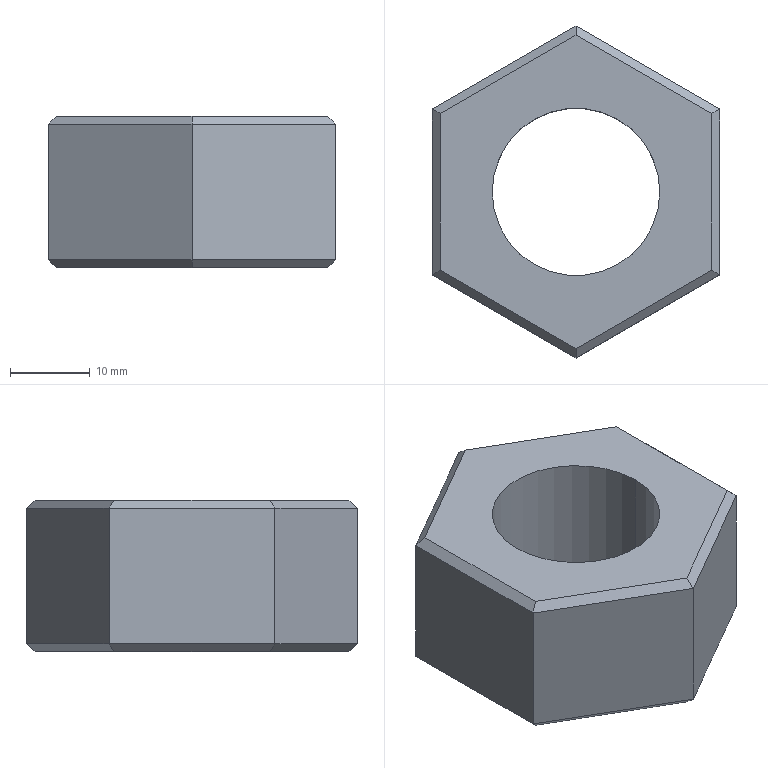Part | STEP file | GLSJ-10-36 | 1 solid | 22 faces | box 36 x 41.569 x 19 mm | volume 14622 mm3 | plane 20 | cylinder 2 | commonest cylinder face diameters 21 x2
STEP:
#1=CARTESIAN_POINT('',(0.,0.,0.));
#2=DIRECTION('',(0.,0.,1.));
#3=DIRECTION('',(1.,0.,0.));
#4=AXIS2_PLACEMENT_3D('',#1,#2,#3);
#5=CARTESIAN_POINT('',(10.5,0.,0.));
#6=VERTEX_POINT('',#5);
#7=CARTESIAN_POINT('',(10.5,0.,19.));
#8=VERTEX_POINT('',#7);
#9=CARTESIAN_POINT('',(10.5,0.,19.));
#10=DIRECTION('',(0.,0.,1.));
#11=VECTOR('',#10,1.);
#12=LINE('',#9,#11);
#13=CARTESIAN_POINT('',(0.,0.,19.));
#14=DIRECTION('',(0.,0.,1.));
#15=DIRECTION('',(1.,0.,0.));
#16=AXIS2_PLACEMENT_3D('',#13,#14,#15);
#17=CYLINDRICAL_SURFACE('',#16,10.5);
#18=CARTESIAN_POINT('',(6.283,0.));
#19=DIRECTION('',(0.,1.));
#20=VECTOR('',#19,1.);
#21=LINE('',#18,#20);
#22=(GEOMETRIC_REPRESENTATION_CONTEXT(2)PARAMETRIC_REPRESENTATION_CONTEXT()REPRESENTATION_CONTEXT('',''));
#23=DEFINITIONAL_REPRESENTATION('',(#21),#22);
#24=PCURVE('',#17,#23);
#25=CARTESIAN_POINT('',(0.,0.,19.));
#26=DIRECTION('',(0.,0.,1.));
#27=DIRECTION('',(1.,0.,0.));
#28=AXIS2_PLACEMENT_3D('',#25,#26,#27);
#29=CYLINDRICAL_SURFACE('',#28,10.5);
#30=CARTESIAN_POINT('',(0.,0.));
#31=DIRECTION('',(0.,1.));
#32=VECTOR('',#31,1.);
#33=LINE('',#30,#32);
#34=(GEOMETRIC_REPRESENTATION_CONTEXT(2)PARAMETRIC_REPRESENTATION_CONTEXT()REPRESENTATION_CONTEXT('',''));
#35=DEFINITIONAL_REPRESENTATION('',(#33),#34);
#36=PCURVE('',#29,#35);
#37=SURFACE_CURVE('',#12,(#24,#36),.PCURVE_S1.);
#38=EDGE_CURVE('',#6,#8,#37,.T.);
#39=ORIENTED_EDGE('',*,*,#38,.T.);
#40=CARTESIAN_POINT('',(-10.5,0.,19.));
#41=VERTEX_POINT('',#40);
#42=CARTESIAN_POINT('',(0.,0.,19.));
#43=DIRECTION('',(0.,0.,1.));
#44=DIRECTION('',(1.,0.,0.));
#45=AXIS2_PLACEMENT_3D('',#42,#43,#44);
#46=CIRCLE('',#45,10.5);
#47=CARTESIAN_POINT('',(0.,0.));
#48=DIRECTION('',(1.,0.));
#49=VECTOR('',#48,1.);
#50=LINE('',#47,#49);
#51=(GEOMETRIC_REPRESENTATION_CONTEXT(2)PARAMETRIC_REPRESENTATION_CONTEXT()REPRESENTATION_CONTEXT('',''));
#52=DEFINITIONAL_REPRESENTATION('',(#50),#51);
#53=PCURVE('',#17,#52);
#54=CARTESIAN_POINT('',(0.,0.,19.));
#55=DIRECTION('',(0.,0.,1.));
#56=DIRECTION('',(1.,0.,0.));
#57=AXIS2_PLACEMENT_3D('',#54,#55,#56);
#58=PLANE('',#57);
#59=CARTESIAN_POINT('',(0.,0.));
#60=DIRECTION('',(1.,0.));
#61=AXIS2_PLACEMENT_2D('',#59,#60);
#62=CIRCLE('',#61,10.5);
#63=(GEOMETRIC_REPRESENTATION_CONTEXT(2)PARAMETRIC_REPRESENTATION_CONTEXT()REPRESENTATION_CONTEXT('',''));
#64=DEFINITIONAL_REPRESENTATION('',(#62),#63);
#65=PCURVE('',#58,#64);
#66=SURFACE_CURVE('',#46,(#53,#65),.PCURVE_S1.);
#67=EDGE_CURVE('',#41,#8,#66,.T.);
#68=ORIENTED_EDGE('',*,*,#67,.F.);
#69=CARTESIAN_POINT('',(-10.5,0.,0.));
#70=VERTEX_POINT('',#69);
#71=CARTESIAN_POINT('',(-10.5,0.,19.));
#72=DIRECTION('',(0.,0.,1.));
#73=VECTOR('',#72,1.);
#74=LINE('',#71,#73);
#75=CARTESIAN_POINT('',(3.142,0.));
#76=DIRECTION('',(0.,1.));
#77=VECTOR('',#76,1.);
#78=LINE('',#75,#77);
#79=(GEOMETRIC_REPRESENTATION_CONTEXT(2)PARAMETRIC_REPRESENTATION_CONTEXT()REPRESENTATION_CONTEXT('',''));
#80=DEFINITIONAL_REPRESENTATION('',(#78),#79);
#81=PCURVE('',#17,#80);
#82=CARTESIAN_POINT('',(3.142,0.));
#83=DIRECTION('',(0.,1.));
#84=VECTOR('',#83,1.);
#85=LINE('',#82,#84);
#86=(GEOMETRIC_REPRESENTATION_CONTEXT(2)PARAMETRIC_REPRESENTATION_CONTEXT()REPRESENTATION_CONTEXT('',''));
#87=DEFINITIONAL_REPRESENTATION('',(#85),#86);
#88=PCURVE('',#29,#87);
#89=SURFACE_CURVE('',#74,(#81,#88),.PCURVE_S1.);
#90=EDGE_CURVE('',#70,#41,#89,.T.);
#91=ORIENTED_EDGE('',*,*,#90,.F.);
#92=CARTESIAN_POINT('',(0.,0.,0.));
#93=DIRECTION('',(0.,0.,1.));
#94=DIRECTION('',(1.,0.,0.));
#95=AXIS2_PLACEMENT_3D('',#92,#93,#94);
#96=CIRCLE('',#95,10.5);
#97=CARTESIAN_POINT('',(0.,-19.));
#98=DIRECTION('',(1.,0.));
#99=VECTOR('',#98,1.);
#100=LINE('',#97,#99);
#101=(GEOMETRIC_REPRESENTATION_CONTEXT(2)PARAMETRIC_REPRESENTATION_CONTEXT()REPRESENTATION_CONTEXT('',''));
#102=DEFINITIONAL_REPRESENTATION('',(#100),#101);
#103=PCURVE('',#17,#102);
#104=CARTESIAN_POINT('',(0.,0.,0.));
#105=DIRECTION('',(0.,0.,1.));
#106=DIRECTION('',(1.,0.,0.));
#107=AXIS2_PLACEMENT_3D('',#104,#105,#106);
#108=PLANE('',#107);
#109=CARTESIAN_POINT('',(0.,0.));
#110=DIRECTION('',(1.,0.));
#111=AXIS2_PLACEMENT_2D('',#109,#110);
#112=CIRCLE('',#111,10.5);
#113=(GEOMETRIC_REPRESENTATION_CONTEXT(2)PARAMETRIC_REPRESENTATION_CONTEXT()REPRESENTATION_CONTEXT('',''));
#114=DEFINITIONAL_REPRESENTATION('',(#112),#113);
#115=PCURVE('',#108,#114);
#116=SURFACE_CURVE('',#96,(#103,#115),.PCURVE_S1.);
#117=EDGE_CURVE('',#70,#6,#116,.T.);
#118=ORIENTED_EDGE('',*,*,#117,.T.);
#119=EDGE_LOOP('',(#39,#68,#91,#118));
#120=FACE_BOUND('',#119,.F.);
#121=ADVANCED_FACE('',(#120),#17,.F.);
#122=CARTESIAN_POINT('',(-18.,10.392,18.));
#123=VERTEX_POINT('',#122);
#124=CARTESIAN_POINT('',(-18.,10.392,1.));
#125=VERTEX_POINT('',#124);
#126=CARTESIAN_POINT('',(-18.,10.392,19.));
#127=DIRECTION('',(0.,0.,-1.));
#128=VECTOR('',#127,1.);
#129=LINE('',#126,#128);
#130=CARTESIAN_POINT('',(-18.,10.392,19.));
#131=DIRECTION('',(1.,0.,0.));
#132=DIRECTION('',(0.,0.,-1.));
#133=AXIS2_PLACEMENT_3D('',#130,#131,#132);
#134=PLANE('',#133);
#135=CARTESIAN_POINT('',(0.,0.));
#136=DIRECTION('',(1.,0.));
#137=VECTOR('',#136,1.);
#138=LINE('',#135,#137);
#139=(GEOMETRIC_REPRESENTATION_CONTEXT(2)PARAMETRIC_REPRESENTATION_CONTEXT()REPRESENTATION_CONTEXT('',''));
#140=DEFINITIONAL_REPRESENTATION('',(#138),#139);
#141=PCURVE('',#134,#140);
#142=CARTESIAN_POINT('',(0.,20.785,19.));
#143=DIRECTION('',(0.5,-0.866,0.));
#144=DIRECTION('',(0.866,0.5,0.));
#145=AXIS2_PLACEMENT_3D('',#142,#143,#144);
#146=PLANE('',#145);
#147=CARTESIAN_POINT('',(-20.785,0.));
#148=DIRECTION('',(0.,-1.));
#149=VECTOR('',#148,1.);
#150=LINE('',#147,#149);
#151=(GEOMETRIC_REPRESENTATION_CONTEXT(2)PARAMETRIC_REPRESENTATION_CONTEXT()REPRESENTATION_CONTEXT('',''));
#152=DEFINITIONAL_REPRESENTATION('',(#150),#151);
#153=PCURVE('',#146,#152);
#154=SURFACE_CURVE('',#129,(#141,#153),.PCURVE_S1.);
#155=EDGE_CURVE('',#123,#125,#154,.T.);
#156=ORIENTED_EDGE('',*,*,#155,.T.);
#157=CARTESIAN_POINT('',(-18.,-10.392,1.));
#158=VERTEX_POINT('',#157);
#159=CARTESIAN_POINT('',(-18.,10.392,1.));
#160=DIRECTION('',(0.,-1.,0.));
#161=VECTOR('',#160,1.);
#162=LINE('',#159,#161);
#163=CARTESIAN_POINT('',(18.,0.));
#164=DIRECTION('',(0.,-1.));
#165=VECTOR('',#164,1.);
#166=LINE('',#163,#165);
#167=(GEOMETRIC_REPRESENTATION_CONTEXT(2)PARAMETRIC_REPRESENTATION_CONTEXT()REPRESENTATION_CONTEXT('',''));
#168=DEFINITIONAL_REPRESENTATION('',(#166),#167);
#169=PCURVE('',#134,#168);
#170=CARTESIAN_POINT('',(-18.,10.392,1.));
#171=DIRECTION('',(0.7071,0.,0.7071));
#172=DIRECTION('',(0.,-1.,0.));
#173=AXIS2_PLACEMENT_3D('',#170,#171,#172);
#174=PLANE('',#173);
#175=CARTESIAN_POINT('',(0.,0.));
#176=DIRECTION('',(1.,0.));
#177=VECTOR('',#176,1.);
#178=LINE('',#175,#177);
#179=(GEOMETRIC_REPRESENTATION_CONTEXT(2)PARAMETRIC_REPRESENTATION_CONTEXT()REPRESENTATION_CONTEXT('',''));
#180=DEFINITIONAL_REPRESENTATION('',(#178),#179);
#181=PCURVE('',#174,#180);
#182=SURFACE_CURVE('',#162,(#169,#181),.PCURVE_S1.);
#183=EDGE_CURVE('',#125,#158,#182,.T.);
#184=ORIENTED_EDGE('',*,*,#183,.T.);
#185=CARTESIAN_POINT('',(-18.,-10.392,18.));
#186=VERTEX_POINT('',#185);
#187=CARTESIAN_POINT('',(-18.,-10.392,19.));
#188=DIRECTION('',(0.,0.,-1.));
#189=VECTOR('',#188,1.);
#190=LINE('',#187,#189);
#191=CARTESIAN_POINT('',(0.,-20.785));
#192=DIRECTION('',(1.,0.));
#193=VECTOR('',#192,1.);
#194=LINE('',#191,#193);
#195=(GEOMETRIC_REPRESENTATION_CONTEXT(2)PARAMETRIC_REPRESENTATION_CONTEXT()REPRESENTATION_CONTEXT('',''));
#196=DEFINITIONAL_REPRESENTATION('',(#194),#195);
#197=PCURVE('',#134,#196);
#198=CARTESIAN_POINT('',(-18.,-10.392,19.));
#199=DIRECTION('',(0.5,0.866,0.));
#200=DIRECTION('',(-0.866,0.5,0.));
#201=AXIS2_PLACEMENT_3D('',#198,#199,#200);
#202=PLANE('',#201);
#203=CARTESIAN_POINT('',(0.,0.));
#204=DIRECTION('',(0.,-1.));
#205=VECTOR('',#204,1.);
#206=LINE('',#203,#205);
#207=(GEOMETRIC_REPRESENTATION_CONTEXT(2)PARAMETRIC_REPRESENTATION_CONTEXT()REPRESENTATION_CONTEXT('',''));
#208=DEFINITIONAL_REPRESENTATION('',(#206),#207);
#209=PCURVE('',#202,#208);
#210=SURFACE_CURVE('',#190,(#197,#209),.PCURVE_S1.);
#211=EDGE_CURVE('',#186,#158,#210,.T.);
#212=ORIENTED_EDGE('',*,*,#211,.F.);
#213=CARTESIAN_POINT('',(-18.,10.392,18.));
#214=DIRECTION('',(0.,1.,0.));
#215=VECTOR('',#214,1.);
#216=LINE('',#213,#215);
#217=CARTESIAN_POINT('',(1.,0.));
#218=DIRECTION('',(0.,1.));
#219=VECTOR('',#218,1.);
#220=LINE('',#217,#219);
#221=(GEOMETRIC_REPRESENTATION_CONTEXT(2)PARAMETRIC_REPRESENTATION_CONTEXT()REPRESENTATION_CONTEXT('',''));
#222=DEFINITIONAL_REPRESENTATION('',(#220),#221);
#223=PCURVE('',#134,#222);
#224=CARTESIAN_POINT('',(-17.,0.,19.));
#225=DIRECTION('',(-0.7071,0.,0.7071));
#226=DIRECTION('',(0.,1.,0.));
#227=AXIS2_PLACEMENT_3D('',#224,#225,#226);
#228=PLANE('',#227);
#229=CARTESIAN_POINT('',(10.392,1.414));
#230=DIRECTION('',(1.,0.));
#231=VECTOR('',#230,1.);
#232=LINE('',#229,#231);
#233=(GEOMETRIC_REPRESENTATION_CONTEXT(2)PARAMETRIC_REPRESENTATION_CONTEXT()REPRESENTATION_CONTEXT('',''));
#234=DEFINITIONAL_REPRESENTATION('',(#232),#233);
#235=PCURVE('',#228,#234);
#236=SURFACE_CURVE('',#216,(#223,#235),.PCURVE_S1.);
#237=EDGE_CURVE('',#186,#123,#236,.T.);
#238=ORIENTED_EDGE('',*,*,#237,.T.);
#239=EDGE_LOOP('',(#156,#184,#212,#238));
#240=FACE_BOUND('',#239,.T.);
#241=ADVANCED_FACE('',(#240),#134,.F.);
#242=ORIENTED_EDGE('',*,*,#211,.T.);
#243=CARTESIAN_POINT('',(0.,-20.785,1.));
#244=VERTEX_POINT('',#243);
#245=CARTESIAN_POINT('',(-18.,-10.392,1.));
#246=DIRECTION('',(0.866,-0.5,0.));
#247=VECTOR('',#246,1.);
#248=LINE('',#245,#247);
#249=CARTESIAN_POINT('',(0.,-18.));
#250=DIRECTION('',(-1.,0.));
#251=VECTOR('',#250,1.);
#252=LINE('',#249,#251);
#253=(GEOMETRIC_REPRESENTATION_CONTEXT(2)PARAMETRIC_REPRESENTATION_CONTEXT()REPRESENTATION_CONTEXT('',''));
#254=DEFINITIONAL_REPRESENTATION('',(#252),#253);
#255=PCURVE('',#202,#254);
#256=CARTESIAN_POINT('',(-18.,-10.392,1.));
#257=DIRECTION('',(0.3536,0.6124,0.7071));
#258=DIRECTION('',(0.866,-0.5,0.));
#259=AXIS2_PLACEMENT_3D('',#256,#257,#258);
#260=PLANE('',#259);
#261=CARTESIAN_POINT('',(0.,0.));
#262=DIRECTION('',(1.,0.));
#263=VECTOR('',#262,1.);
#264=LINE('',#261,#263);
#265=(GEOMETRIC_REPRESENTATION_CONTEXT(2)PARAMETRIC_REPRESENTATION_CONTEXT()REPRESENTATION_CONTEXT('',''));
#266=DEFINITIONAL_REPRESENTATION('',(#264),#265);
#267=PCURVE('',#260,#266);
#268=SURFACE_CURVE('',#248,(#255,#267),.PCURVE_S1.);
#269=EDGE_CURVE('',#158,#244,#268,.T.);
#270=ORIENTED_EDGE('',*,*,#269,.T.);
#271=CARTESIAN_POINT('',(0.,-20.785,18.));
#272=VERTEX_POINT('',#271);
#273=CARTESIAN_POINT('',(0.,-20.785,19.));
#274=DIRECTION('',(0.,0.,-1.));
#275=VECTOR('',#274,1.);
#276=LINE('',#273,#275);
#277=CARTESIAN_POINT('',(-20.785,0.));
#278=DIRECTION('',(0.,-1.));
#279=VECTOR('',#278,1.);
#280=LINE('',#277,#279);
#281=(GEOMETRIC_REPRESENTATION_CONTEXT(2)PARAMETRIC_REPRESENTATION_CONTEXT()REPRESENTATION_CONTEXT('',''));
#282=DEFINITIONAL_REPRESENTATION('',(#280),#281);
#283=PCURVE('',#202,#282);
#284=CARTESIAN_POINT('',(0.,-20.785,19.));
#285=DIRECTION('',(-0.5,0.866,0.));
#286=DIRECTION('',(-0.866,-0.5,0.));
#287=AXIS2_PLACEMENT_3D('',#284,#285,#286);
#288=PLANE('',#287);
#289=CARTESIAN_POINT('',(0.,0.));
#290=DIRECTION('',(0.,-1.));
#291=VECTOR('',#290,1.);
#292=LINE('',#289,#291);
#293=(GEOMETRIC_REPRESENTATION_CONTEXT(2)PARAMETRIC_REPRESENTATION_CONTEXT()REPRESENTATION_CONTEXT('',''));
#294=DEFINITIONAL_REPRESENTATION('',(#292),#293);
#295=PCURVE('',#288,#294);
#296=SURFACE_CURVE('',#276,(#283,#295),.PCURVE_S1.);
#297=EDGE_CURVE('',#272,#244,#296,.T.);
#298=ORIENTED_EDGE('',*,*,#297,.F.);
#299=CARTESIAN_POINT('',(-18.,-10.392,18.));
#300=DIRECTION('',(-0.866,0.5,0.));
#301=VECTOR('',#300,1.);
#302=LINE('',#299,#301);
#303=CARTESIAN_POINT('',(0.,-1.));
#304=DIRECTION('',(1.,0.));
#305=VECTOR('',#304,1.);
#306=LINE('',#303,#305);
#307=(GEOMETRIC_REPRESENTATION_CONTEXT(2)PARAMETRIC_REPRESENTATION_CONTEXT()REPRESENTATION_CONTEXT('',''));
#308=DEFINITIONAL_REPRESENTATION('',(#306),#307);
#309=PCURVE('',#202,#308);
#310=CARTESIAN_POINT('',(-8.5,-14.722,19.));
#311=DIRECTION('',(-0.3536,-0.6124,0.7071));
#312=DIRECTION('',(-0.866,0.5,0.));
#313=AXIS2_PLACEMENT_3D('',#310,#311,#312);
#314=PLANE('',#313);
#315=CARTESIAN_POINT('',(10.392,1.414));
#316=DIRECTION('',(1.,0.));
#317=VECTOR('',#316,1.);
#318=LINE('',#315,#317);
#319=(GEOMETRIC_REPRESENTATION_CONTEXT(2)PARAMETRIC_REPRESENTATION_CONTEXT()REPRESENTATION_CONTEXT('',''));
#320=DEFINITIONAL_REPRESENTATION('',(#318),#319);
#321=PCURVE('',#314,#320);
#322=SURFACE_CURVE('',#302,(#309,#321),.PCURVE_S1.);
#323=EDGE_CURVE('',#272,#186,#322,.T.);
#324=ORIENTED_EDGE('',*,*,#323,.T.);
#325=EDGE_LOOP('',(#242,#270,#298,#324));
#326=FACE_BOUND('',#325,.T.);
#327=ADVANCED_FACE('',(#326),#202,.F.);
#328=ORIENTED_EDGE('',*,*,#297,.T.);
#329=CARTESIAN_POINT('',(18.,-10.392,1.));
#330=VERTEX_POINT('',#329);
#331=CARTESIAN_POINT('',(0.,-20.785,1.));
#332=DIRECTION('',(0.866,0.5,0.));
#333=VECTOR('',#332,1.);
#334=LINE('',#331,#333);
#335=CARTESIAN_POINT('',(0.,-18.));
#336=DIRECTION('',(-1.,0.));
#337=VECTOR('',#336,1.);
#338=LINE('',#335,#337);
#339=(GEOMETRIC_REPRESENTATION_CONTEXT(2)PARAMETRIC_REPRESENTATION_CONTEXT()REPRESENTATION_CONTEXT('',''));
#340=DEFINITIONAL_REPRESENTATION('',(#338),#339);
#341=PCURVE('',#288,#340);
#342=CARTESIAN_POINT('',(0.,-20.785,1.));
#343=DIRECTION('',(-0.3536,0.6124,0.7071));
#344=DIRECTION('',(0.866,0.5,0.));
#345=AXIS2_PLACEMENT_3D('',#342,#343,#344);
#346=PLANE('',#345);
#347=CARTESIAN_POINT('',(0.,0.));
#348=DIRECTION('',(1.,0.));
#349=VECTOR('',#348,1.);
#350=LINE('',#347,#349);
#351=(GEOMETRIC_REPRESENTATION_CONTEXT(2)PARAMETRIC_REPRESENTATION_CONTEXT()REPRESENTATION_CONTEXT('',''));
#352=DEFINITIONAL_REPRESENTATION('',(#350),#351);
#353=PCURVE('',#346,#352);
#354=SURFACE_CURVE('',#334,(#341,#353),.PCURVE_S1.);
#355=EDGE_CURVE('',#244,#330,#354,.T.);
#356=ORIENTED_EDGE('',*,*,#355,.T.);
#357=CARTESIAN_POINT('',(18.,-10.392,18.));
#358=VERTEX_POINT('',#357);
#359=CARTESIAN_POINT('',(18.,-10.392,19.));
#360=DIRECTION('',(0.,0.,-1.));
#361=VECTOR('',#360,1.);
#362=LINE('',#359,#361);
#363=CARTESIAN_POINT('',(-20.785,0.));
#364=DIRECTION('',(0.,-1.));
#365=VECTOR('',#364,1.);
#366=LINE('',#363,#365);
#367=(GEOMETRIC_REPRESENTATION_CONTEXT(2)PARAMETRIC_REPRESENTATION_CONTEXT()REPRESENTATION_CONTEXT('',''));
#368=DEFINITIONAL_REPRESENTATION('',(#366),#367);
#369=PCURVE('',#288,#368);
#370=CARTESIAN_POINT('',(18.,-10.392,19.));
#371=DIRECTION('',(-1.,0.,0.));
#372=DIRECTION('',(0.,-1.,0.));
#373=AXIS2_PLACEMENT_3D('',#370,#371,#372);
#374=PLANE('',#373);
#375=CARTESIAN_POINT('',(0.,0.));
#376=DIRECTION('',(0.,-1.));
#377=VECTOR('',#376,1.);
#378=LINE('',#375,#377);
#379=(GEOMETRIC_REPRESENTATION_CONTEXT(2)PARAMETRIC_REPRESENTATION_CONTEXT()REPRESENTATION_CONTEXT('',''));
#380=DEFINITIONAL_REPRESENTATION('',(#378),#379);
#381=PCURVE('',#374,#380);
#382=SURFACE_CURVE('',#362,(#369,#381),.PCURVE_S1.);
#383=EDGE_CURVE('',#358,#330,#382,.T.);
#384=ORIENTED_EDGE('',*,*,#383,.F.);
#385=CARTESIAN_POINT('',(0.,-20.785,18.));
#386=DIRECTION('',(-0.866,-0.5,0.));
#387=VECTOR('',#386,1.);
#388=LINE('',#385,#387);
#389=CARTESIAN_POINT('',(0.,-1.));
#390=DIRECTION('',(1.,0.));
#391=VECTOR('',#390,1.);
#392=LINE('',#389,#391);
#393=(GEOMETRIC_REPRESENTATION_CONTEXT(2)PARAMETRIC_REPRESENTATION_CONTEXT()REPRESENTATION_CONTEXT('',''));
#394=DEFINITIONAL_REPRESENTATION('',(#392),#393);
#395=PCURVE('',#288,#394);
#396=CARTESIAN_POINT('',(8.5,-14.722,19.));
#397=DIRECTION('',(0.3536,-0.6124,0.7071));
#398=DIRECTION('',(-0.866,-0.5,0.));
#399=AXIS2_PLACEMENT_3D('',#396,#397,#398);
#400=PLANE('',#399);
#401=CARTESIAN_POINT('',(10.392,1.414));
#402=DIRECTION('',(1.,0.));
#403=VECTOR('',#402,1.);
#404=LINE('',#401,#403);
#405=(GEOMETRIC_REPRESENTATION_CONTEXT(2)PARAMETRIC_REPRESENTATION_CONTEXT()REPRESENTATION_CONTEXT('',''));
#406=DEFINITIONAL_REPRESENTATION('',(#404),#405);
#407=PCURVE('',#400,#406);
#408=SURFACE_CURVE('',#388,(#395,#407),.PCURVE_S1.);
#409=EDGE_CURVE('',#358,#272,#408,.T.);
#410=ORIENTED_EDGE('',*,*,#409,.T.);
#411=EDGE_LOOP('',(#328,#356,#384,#410));
#412=FACE_BOUND('',#411,.T.);
#413=ADVANCED_FACE('',(#412),#288,.F.);
#414=ORIENTED_EDGE('',*,*,#383,.T.);
#415=CARTESIAN_POINT('',(18.,10.392,1.));
#416=VERTEX_POINT('',#415);
#417=CARTESIAN_POINT('',(18.,-10.392,1.));
#418=DIRECTION('',(0.,1.,0.));
#419=VECTOR('',#418,1.);
#420=LINE('',#417,#419);
#421=CARTESIAN_POINT('',(0.,-18.));
#422=DIRECTION('',(-1.,0.));
#423=VECTOR('',#422,1.);
#424=LINE('',#421,#423);
#425=(GEOMETRIC_REPRESENTATION_CONTEXT(2)PARAMETRIC_REPRESENTATION_CONTEXT()REPRESENTATION_CONTEXT('',''));
#426=DEFINITIONAL_REPRESENTATION('',(#424),#425);
#427=PCURVE('',#374,#426);
#428=CARTESIAN_POINT('',(18.,-10.392,1.));
#429=DIRECTION('',(-0.7071,0.,0.7071));
#430=DIRECTION('',(0.,1.,0.));
#431=AXIS2_PLACEMENT_3D('',#428,#429,#430);
#432=PLANE('',#431);
#433=CARTESIAN_POINT('',(0.,0.));
#434=DIRECTION('',(1.,0.));
#435=VECTOR('',#434,1.);
#436=LINE('',#433,#435);
#437=(GEOMETRIC_REPRESENTATION_CONTEXT(2)PARAMETRIC_REPRESENTATION_CONTEXT()REPRESENTATION_CONTEXT('',''));
#438=DEFINITIONAL_REPRESENTATION('',(#436),#437);
#439=PCURVE('',#432,#438);
#440=SURFACE_CURVE('',#420,(#427,#439),.PCURVE_S1.);
#441=EDGE_CURVE('',#330,#416,#440,.T.);
#442=ORIENTED_EDGE('',*,*,#441,.T.);
#443=CARTESIAN_POINT('',(18.,10.392,18.));
#444=VERTEX_POINT('',#443);
#445=CARTESIAN_POINT('',(18.,10.392,19.));
#446=DIRECTION('',(0.,0.,-1.));
#447=VECTOR('',#446,1.);
#448=LINE('',#445,#447);
#449=CARTESIAN_POINT('',(-20.785,0.));
#450=DIRECTION('',(0.,-1.));
#451=VECTOR('',#450,1.);
#452=LINE('',#449,#451);
#453=(GEOMETRIC_REPRESENTATION_CONTEXT(2)PARAMETRIC_REPRESENTATION_CONTEXT()REPRESENTATION_CONTEXT('',''));
#454=DEFINITIONAL_REPRESENTATION('',(#452),#453);
#455=PCURVE('',#374,#454);
#456=CARTESIAN_POINT('',(18.,10.392,19.));
#457=DIRECTION('',(-0.5,-0.866,0.));
#458=DIRECTION('',(0.866,-0.5,0.));
#459=AXIS2_PLACEMENT_3D('',#456,#457,#458);
#460=PLANE('',#459);
#461=CARTESIAN_POINT('',(0.,0.));
#462=DIRECTION('',(0.,-1.));
#463=VECTOR('',#462,1.);
#464=LINE('',#461,#463);
#465=(GEOMETRIC_REPRESENTATION_CONTEXT(2)PARAMETRIC_REPRESENTATION_CONTEXT()REPRESENTATION_CONTEXT('',''));
#466=DEFINITIONAL_REPRESENTATION('',(#464),#465);
#467=PCURVE('',#460,#466);
#468=SURFACE_CURVE('',#448,(#455,#467),.PCURVE_S1.);
#469=EDGE_CURVE('',#444,#416,#468,.T.);
#470=ORIENTED_EDGE('',*,*,#469,.F.);
#471=CARTESIAN_POINT('',(18.,-10.392,18.));
#472=DIRECTION('',(0.,-1.,0.));
#473=VECTOR('',#472,1.);
#474=LINE('',#471,#473);
#475=CARTESIAN_POINT('',(0.,-1.));
#476=DIRECTION('',(1.,0.));
#477=VECTOR('',#476,1.);
#478=LINE('',#475,#477);
#479=(GEOMETRIC_REPRESENTATION_CONTEXT(2)PARAMETRIC_REPRESENTATION_CONTEXT()REPRESENTATION_CONTEXT('',''));
#480=DEFINITIONAL_REPRESENTATION('',(#478),#479);
#481=PCURVE('',#374,#480);
#482=CARTESIAN_POINT('',(17.,0.,19.));
#483=DIRECTION('',(0.7071,0.,0.7071));
#484=DIRECTION('',(0.,-1.,0.));
#485=AXIS2_PLACEMENT_3D('',#482,#483,#484);
#486=PLANE('',#485);
#487=CARTESIAN_POINT('',(10.392,1.414));
#488=DIRECTION('',(1.,0.));
#489=VECTOR('',#488,1.);
#490=LINE('',#487,#489);
#491=(GEOMETRIC_REPRESENTATION_CONTEXT(2)PARAMETRIC_REPRESENTATION_CONTEXT()REPRESENTATION_CONTEXT('',''));
#492=DEFINITIONAL_REPRESENTATION('',(#490),#491);
#493=PCURVE('',#486,#492);
#494=SURFACE_CURVE('',#474,(#481,#493),.PCURVE_S1.);
#495=EDGE_CURVE('',#444,#358,#494,.T.);
#496=ORIENTED_EDGE('',*,*,#495,.T.);
#497=EDGE_LOOP('',(#414,#442,#470,#496));
#498=FACE_BOUND('',#497,.T.);
#499=ADVANCED_FACE('',(#498),#374,.F.);
#500=ORIENTED_EDGE('',*,*,#469,.T.);
#501=CARTESIAN_POINT('',(0.,20.785,1.));
#502=VERTEX_POINT('',#501);
#503=CARTESIAN_POINT('',(18.,10.392,1.));
#504=DIRECTION('',(-0.866,0.5,0.));
#505=VECTOR('',#504,1.);
#506=LINE('',#503,#505);
#507=CARTESIAN_POINT('',(0.,-18.));
#508=DIRECTION('',(-1.,0.));
#509=VECTOR('',#508,1.);
#510=LINE('',#507,#509);
#511=(GEOMETRIC_REPRESENTATION_CONTEXT(2)PARAMETRIC_REPRESENTATION_CONTEXT()REPRESENTATION_CONTEXT('',''));
#512=DEFINITIONAL_REPRESENTATION('',(#510),#511);
#513=PCURVE('',#460,#512);
#514=CARTESIAN_POINT('',(18.,10.392,1.));
#515=DIRECTION('',(-0.3536,-0.6124,0.7071));
#516=DIRECTION('',(-0.866,0.5,0.));
#517=AXIS2_PLACEMENT_3D('',#514,#515,#516);
#518=PLANE('',#517);
#519=CARTESIAN_POINT('',(0.,0.));
#520=DIRECTION('',(1.,0.));
#521=VECTOR('',#520,1.);
#522=LINE('',#519,#521);
#523=(GEOMETRIC_REPRESENTATION_CONTEXT(2)PARAMETRIC_REPRESENTATION_CONTEXT()REPRESENTATION_CONTEXT('',''));
#524=DEFINITIONAL_REPRESENTATION('',(#522),#523);
#525=PCURVE('',#518,#524);
#526=SURFACE_CURVE('',#506,(#513,#525),.PCURVE_S1.);
#527=EDGE_CURVE('',#416,#502,#526,.T.);
#528=ORIENTED_EDGE('',*,*,#527,.T.);
#529=CARTESIAN_POINT('',(0.,20.785,18.));
#530=VERTEX_POINT('',#529);
#531=CARTESIAN_POINT('',(0.,20.785,19.));
#532=DIRECTION('',(0.,0.,-1.));
#533=VECTOR('',#532,1.);
#534=LINE('',#531,#533);
#535=CARTESIAN_POINT('',(-20.785,0.));
#536=DIRECTION('',(0.,-1.));
#537=VECTOR('',#536,1.);
#538=LINE('',#535,#537);
#539=(GEOMETRIC_REPRESENTATION_CONTEXT(2)PARAMETRIC_REPRESENTATION_CONTEXT()REPRESENTATION_CONTEXT('',''));
#540=DEFINITIONAL_REPRESENTATION('',(#538),#539);
#541=PCURVE('',#460,#540);
#542=CARTESIAN_POINT('',(0.,0.));
#543=DIRECTION('',(0.,-1.));
#544=VECTOR('',#543,1.);
#545=LINE('',#542,#544);
#546=(GEOMETRIC_REPRESENTATION_CONTEXT(2)PARAMETRIC_REPRESENTATION_CONTEXT()REPRESENTATION_CONTEXT('',''));
#547=DEFINITIONAL_REPRESENTATION('',(#545),#546);
#548=PCURVE('',#146,#547);
#549=SURFACE_CURVE('',#534,(#541,#548),.PCURVE_S1.);
#550=EDGE_CURVE('',#530,#502,#549,.T.);
#551=ORIENTED_EDGE('',*,*,#550,.F.);
#552=CARTESIAN_POINT('',(18.,10.392,18.));
#553=DIRECTION('',(0.866,-0.5,0.));
#554=VECTOR('',#553,1.);
#555=LINE('',#552,#554);
#556=CARTESIAN_POINT('',(0.,-1.));
#557=DIRECTION('',(1.,0.));
#558=VECTOR('',#557,1.);
#559=LINE('',#556,#558);
#560=(GEOMETRIC_REPRESENTATION_CONTEXT(2)PARAMETRIC_REPRESENTATION_CONTEXT()REPRESENTATION_CONTEXT('',''));
#561=DEFINITIONAL_REPRESENTATION('',(#559),#560);
#562=PCURVE('',#460,#561);
#563=CARTESIAN_POINT('',(8.5,14.722,19.));
#564=DIRECTION('',(0.3536,0.6124,0.7071));
#565=DIRECTION('',(0.866,-0.5,0.));
#566=AXIS2_PLACEMENT_3D('',#563,#564,#565);
#567=PLANE('',#566);
#568=CARTESIAN_POINT('',(10.392,1.414));
#569=DIRECTION('',(1.,0.));
#570=VECTOR('',#569,1.);
#571=LINE('',#568,#570);
#572=(GEOMETRIC_REPRESENTATION_CONTEXT(2)PARAMETRIC_REPRESENTATION_CONTEXT()REPRESENTATION_CONTEXT('',''));
#573=DEFINITIONAL_REPRESENTATION('',(#571),#572);
#574=PCURVE('',#567,#573);
#575=SURFACE_CURVE('',#555,(#562,#574),.PCURVE_S1.);
#576=EDGE_CURVE('',#530,#444,#575,.T.);
#577=ORIENTED_EDGE('',*,*,#576,.T.);
#578=EDGE_LOOP('',(#500,#528,#551,#577));
#579=FACE_BOUND('',#578,.T.);
#580=ADVANCED_FACE('',(#579),#460,.F.);
#581=ORIENTED_EDGE('',*,*,#550,.T.);
#582=CARTESIAN_POINT('',(0.,20.785,1.));
#583=DIRECTION('',(-0.866,-0.5,0.));
#584=VECTOR('',#583,1.);
#585=LINE('',#582,#584);
#586=CARTESIAN_POINT('',(0.,-18.));
#587=DIRECTION('',(-1.,0.));
#588=VECTOR('',#587,1.);
#589=LINE('',#586,#588);
#590=(GEOMETRIC_REPRESENTATION_CONTEXT(2)PARAMETRIC_REPRESENTATION_CONTEXT()REPRESENTATION_CONTEXT('',''));
#591=DEFINITIONAL_REPRESENTATION('',(#589),#590);
#592=PCURVE('',#146,#591);
#593=CARTESIAN_POINT('',(0.,20.785,1.));
#594=DIRECTION('',(0.3536,-0.6124,0.7071));
#595=DIRECTION('',(-0.866,-0.5,0.));
#596=AXIS2_PLACEMENT_3D('',#593,#594,#595);
#597=PLANE('',#596);
#598=CARTESIAN_POINT('',(0.,0.));
#599=DIRECTION('',(1.,0.));
#600=VECTOR('',#599,1.);
#601=LINE('',#598,#600);
#602=(GEOMETRIC_REPRESENTATION_CONTEXT(2)PARAMETRIC_REPRESENTATION_CONTEXT()REPRESENTATION_CONTEXT('',''));
#603=DEFINITIONAL_REPRESENTATION('',(#601),#602);
#604=PCURVE('',#597,#603);
#605=SURFACE_CURVE('',#585,(#592,#604),.PCURVE_S1.);
#606=EDGE_CURVE('',#502,#125,#605,.T.);
#607=ORIENTED_EDGE('',*,*,#606,.T.);
#608=ORIENTED_EDGE('',*,*,#155,.F.);
#609=CARTESIAN_POINT('',(0.,20.785,18.));
#610=DIRECTION('',(0.866,0.5,0.));
#611=VECTOR('',#610,1.);
#612=LINE('',#609,#611);
#613=CARTESIAN_POINT('',(0.,-1.));
#614=DIRECTION('',(1.,0.));
#615=VECTOR('',#614,1.);
#616=LINE('',#613,#615);
#617=(GEOMETRIC_REPRESENTATION_CONTEXT(2)PARAMETRIC_REPRESENTATION_CONTEXT()REPRESENTATION_CONTEXT('',''));
#618=DEFINITIONAL_REPRESENTATION('',(#616),#617);
#619=PCURVE('',#146,#618);
#620=CARTESIAN_POINT('',(-8.5,14.722,19.));
#621=DIRECTION('',(-0.3536,0.6124,0.7071));
#622=DIRECTION('',(0.866,0.5,0.));
#623=AXIS2_PLACEMENT_3D('',#620,#621,#622);
#624=PLANE('',#623);
#625=CARTESIAN_POINT('',(10.392,1.414));
#626=DIRECTION('',(1.,0.));
#627=VECTOR('',#626,1.);
#628=LINE('',#625,#627);
#629=(GEOMETRIC_REPRESENTATION_CONTEXT(2)PARAMETRIC_REPRESENTATION_CONTEXT()REPRESENTATION_CONTEXT('',''));
#630=DEFINITIONAL_REPRESENTATION('',(#628),#629);
#631=PCURVE('',#624,#630);
#632=SURFACE_CURVE('',#612,(#619,#631),.PCURVE_S1.);
#633=EDGE_CURVE('',#123,#530,#632,.T.);
#634=ORIENTED_EDGE('',*,*,#633,.T.);
#635=EDGE_LOOP('',(#581,#607,#608,#634));
#636=FACE_BOUND('',#635,.T.);
#637=ADVANCED_FACE('',(#636),#146,.F.);
#638=CARTESIAN_POINT('',(17.,9.815,19.));
#639=VERTEX_POINT('',#638);
#640=CARTESIAN_POINT('',(0.,19.63,19.));
#641=VERTEX_POINT('',#640);
#642=CARTESIAN_POINT('',(-0.5,19.919,19.));
#643=DIRECTION('',(-0.866,0.5,0.));
#644=VECTOR('',#643,1.);
#645=LINE('',#642,#644);
#646=CARTESIAN_POINT('',(-0.5,19.919));
#647=DIRECTION('',(-0.866,0.5));
#648=VECTOR('',#647,1.);
#649=LINE('',#646,#648);
#650=(GEOMETRIC_REPRESENTATION_CONTEXT(2)PARAMETRIC_REPRESENTATION_CONTEXT()REPRESENTATION_CONTEXT('',''));
#651=DEFINITIONAL_REPRESENTATION('',(#649),#650);
#652=PCURVE('',#58,#651);
#653=CARTESIAN_POINT('',(-10.392,0.));
#654=DIRECTION('',(-1.,0.));
#655=VECTOR('',#654,1.);
#656=LINE('',#653,#655);
#657=(GEOMETRIC_REPRESENTATION_CONTEXT(2)PARAMETRIC_REPRESENTATION_CONTEXT()REPRESENTATION_CONTEXT('',''));
#658=DEFINITIONAL_REPRESENTATION('',(#656),#657);
#659=PCURVE('',#567,#658);
#660=SURFACE_CURVE('',#645,(#652,#659),.PCURVE_S1.);
#661=EDGE_CURVE('',#639,#641,#660,.T.);
#662=ORIENTED_EDGE('',*,*,#661,.T.);
#663=CARTESIAN_POINT('',(-17.,9.815,19.));
#664=VERTEX_POINT('',#663);
#665=CARTESIAN_POINT('',(-17.5,9.526,19.));
#666=DIRECTION('',(-0.866,-0.5,0.));
#667=VECTOR('',#666,1.);
#668=LINE('',#665,#667);
#669=CARTESIAN_POINT('',(-17.5,9.526));
#670=DIRECTION('',(-0.866,-0.5));
#671=VECTOR('',#670,1.);
#672=LINE('',#669,#671);
#673=(GEOMETRIC_REPRESENTATION_CONTEXT(2)PARAMETRIC_REPRESENTATION_CONTEXT()REPRESENTATION_CONTEXT('',''));
#674=DEFINITIONAL_REPRESENTATION('',(#672),#673);
#675=PCURVE('',#58,#674);
#676=CARTESIAN_POINT('',(-10.392,0.));
#677=DIRECTION('',(-1.,0.));
#678=VECTOR('',#677,1.);
#679=LINE('',#676,#678);
#680=(GEOMETRIC_REPRESENTATION_CONTEXT(2)PARAMETRIC_REPRESENTATION_CONTEXT()REPRESENTATION_CONTEXT('',''));
#681=DEFINITIONAL_REPRESENTATION('',(#679),#680);
#682=PCURVE('',#624,#681);
#683=SURFACE_CURVE('',#668,(#675,#682),.PCURVE_S1.);
#684=EDGE_CURVE('',#641,#664,#683,.T.);
#685=ORIENTED_EDGE('',*,*,#684,.T.);
#686=CARTESIAN_POINT('',(-17.,-9.815,19.));
#687=VERTEX_POINT('',#686);
#688=CARTESIAN_POINT('',(-17.,-10.392,19.));
#689=DIRECTION('',(0.,-1.,0.));
#690=VECTOR('',#689,1.);
#691=LINE('',#688,#690);
#692=CARTESIAN_POINT('',(-17.,-10.392));
#693=DIRECTION('',(0.,-1.));
#694=VECTOR('',#693,1.);
#695=LINE('',#692,#694);
#696=(GEOMETRIC_REPRESENTATION_CONTEXT(2)PARAMETRIC_REPRESENTATION_CONTEXT()REPRESENTATION_CONTEXT('',''));
#697=DEFINITIONAL_REPRESENTATION('',(#695),#696);
#698=PCURVE('',#58,#697);
#699=CARTESIAN_POINT('',(-10.392,0.));
#700=DIRECTION('',(-1.,0.));
#701=VECTOR('',#700,1.);
#702=LINE('',#699,#701);
#703=(GEOMETRIC_REPRESENTATION_CONTEXT(2)PARAMETRIC_REPRESENTATION_CONTEXT()REPRESENTATION_CONTEXT('',''));
#704=DEFINITIONAL_REPRESENTATION('',(#702),#703);
#705=PCURVE('',#228,#704);
#706=SURFACE_CURVE('',#691,(#698,#705),.PCURVE_S1.);
#707=EDGE_CURVE('',#664,#687,#706,.T.);
#708=ORIENTED_EDGE('',*,*,#707,.T.);
#709=CARTESIAN_POINT('',(0.,-19.63,19.));
#710=VERTEX_POINT('',#709);
#711=CARTESIAN_POINT('',(0.5,-19.919,19.));
#712=DIRECTION('',(0.866,-0.5,0.));
#713=VECTOR('',#712,1.);
#714=LINE('',#711,#713);
#715=CARTESIAN_POINT('',(0.5,-19.919));
#716=DIRECTION('',(0.866,-0.5));
#717=VECTOR('',#716,1.);
#718=LINE('',#715,#717);
#719=(GEOMETRIC_REPRESENTATION_CONTEXT(2)PARAMETRIC_REPRESENTATION_CONTEXT()REPRESENTATION_CONTEXT('',''));
#720=DEFINITIONAL_REPRESENTATION('',(#718),#719);
#721=PCURVE('',#58,#720);
#722=CARTESIAN_POINT('',(-10.392,0.));
#723=DIRECTION('',(-1.,0.));
#724=VECTOR('',#723,1.);
#725=LINE('',#722,#724);
#726=(GEOMETRIC_REPRESENTATION_CONTEXT(2)PARAMETRIC_REPRESENTATION_CONTEXT()REPRESENTATION_CONTEXT('',''));
#727=DEFINITIONAL_REPRESENTATION('',(#725),#726);
#728=PCURVE('',#314,#727);
#729=SURFACE_CURVE('',#714,(#721,#728),.PCURVE_S1.);
#730=EDGE_CURVE('',#687,#710,#729,.T.);
#731=ORIENTED_EDGE('',*,*,#730,.T.);
#732=CARTESIAN_POINT('',(17.,-9.815,19.));
#733=VERTEX_POINT('',#732);
#734=CARTESIAN_POINT('',(17.5,-9.526,19.));
#735=DIRECTION('',(0.866,0.5,0.));
#736=VECTOR('',#735,1.);
#737=LINE('',#734,#736);
#738=CARTESIAN_POINT('',(17.5,-9.526));
#739=DIRECTION('',(0.866,0.5));
#740=VECTOR('',#739,1.);
#741=LINE('',#738,#740);
#742=(GEOMETRIC_REPRESENTATION_CONTEXT(2)PARAMETRIC_REPRESENTATION_CONTEXT()REPRESENTATION_CONTEXT('',''));
#743=DEFINITIONAL_REPRESENTATION('',(#741),#742);
#744=PCURVE('',#58,#743);
#745=CARTESIAN_POINT('',(-10.392,0.));
#746=DIRECTION('',(-1.,0.));
#747=VECTOR('',#746,1.);
#748=LINE('',#745,#747);
#749=(GEOMETRIC_REPRESENTATION_CONTEXT(2)PARAMETRIC_REPRESENTATION_CONTEXT()REPRESENTATION_CONTEXT('',''));
#750=DEFINITIONAL_REPRESENTATION('',(#748),#749);
#751=PCURVE('',#400,#750);
#752=SURFACE_CURVE('',#737,(#744,#751),.PCURVE_S1.);
#753=EDGE_CURVE('',#710,#733,#752,.T.);
#754=ORIENTED_EDGE('',*,*,#753,.T.);
#755=CARTESIAN_POINT('',(17.,10.392,19.));
#756=DIRECTION('',(0.,1.,0.));
#757=VECTOR('',#756,1.);
#758=LINE('',#755,#757);
#759=CARTESIAN_POINT('',(17.,10.392));
#760=DIRECTION('',(0.,1.));
#761=VECTOR('',#760,1.);
#762=LINE('',#759,#761);
#763=(GEOMETRIC_REPRESENTATION_CONTEXT(2)PARAMETRIC_REPRESENTATION_CONTEXT()REPRESENTATION_CONTEXT('',''));
#764=DEFINITIONAL_REPRESENTATION('',(#762),#763);
#765=PCURVE('',#58,#764);
#766=CARTESIAN_POINT('',(-10.392,0.));
#767=DIRECTION('',(-1.,0.));
#768=VECTOR('',#767,1.);
#769=LINE('',#766,#768);
#770=(GEOMETRIC_REPRESENTATION_CONTEXT(2)PARAMETRIC_REPRESENTATION_CONTEXT()REPRESENTATION_CONTEXT('',''));
#771=DEFINITIONAL_REPRESENTATION('',(#769),#770);
#772=PCURVE('',#486,#771);
#773=SURFACE_CURVE('',#758,(#765,#772),.PCURVE_S1.);
#774=EDGE_CURVE('',#733,#639,#773,.T.);
#775=ORIENTED_EDGE('',*,*,#774,.T.);
#776=EDGE_LOOP('',(#662,#685,#708,#731,#754,#775));
#777=FACE_BOUND('',#776,.T.);
#778=CARTESIAN_POINT('',(0.,0.,19.));
#779=DIRECTION('',(0.,0.,1.));
#780=DIRECTION('',(1.,0.,0.));
#781=AXIS2_PLACEMENT_3D('',#778,#779,#780);
#782=CIRCLE('',#781,10.5);
#783=CARTESIAN_POINT('',(0.,0.));
#784=DIRECTION('',(1.,0.));
#785=AXIS2_PLACEMENT_2D('',#783,#784);
#786=CIRCLE('',#785,10.5);
#787=(GEOMETRIC_REPRESENTATION_CONTEXT(2)PARAMETRIC_REPRESENTATION_CONTEXT()REPRESENTATION_CONTEXT('',''));
#788=DEFINITIONAL_REPRESENTATION('',(#786),#787);
#789=PCURVE('',#58,#788);
#790=CARTESIAN_POINT('',(0.,0.));
#791=DIRECTION('',(1.,0.));
#792=VECTOR('',#791,1.);
#793=LINE('',#790,#792);
#794=(GEOMETRIC_REPRESENTATION_CONTEXT(2)PARAMETRIC_REPRESENTATION_CONTEXT()REPRESENTATION_CONTEXT('',''));
#795=DEFINITIONAL_REPRESENTATION('',(#793),#794);
#796=PCURVE('',#29,#795);
#797=SURFACE_CURVE('',#782,(#789,#796),.PCURVE_S1.);
#798=EDGE_CURVE('',#8,#41,#797,.T.);
#799=ORIENTED_EDGE('',*,*,#798,.F.);
#800=ORIENTED_EDGE('',*,*,#67,.F.);
#801=EDGE_LOOP('',(#799,#800));
#802=FACE_BOUND('',#801,.T.);
#803=ADVANCED_FACE('',(#777,#802),#58,.T.);
#804=CARTESIAN_POINT('',(0.,19.63,0.));
#805=VERTEX_POINT('',#804);
#806=CARTESIAN_POINT('',(17.,9.815,0.));
#807=VERTEX_POINT('',#806);
#808=CARTESIAN_POINT('',(8.5,14.722,0.));
#809=DIRECTION('',(0.866,-0.5,0.));
#810=VECTOR('',#809,1.);
#811=LINE('',#808,#810);
#812=CARTESIAN_POINT('',(8.5,14.722));
#813=DIRECTION('',(0.866,-0.5));
#814=VECTOR('',#813,1.);
#815=LINE('',#812,#814);
#816=(GEOMETRIC_REPRESENTATION_CONTEXT(2)PARAMETRIC_REPRESENTATION_CONTEXT()REPRESENTATION_CONTEXT('',''));
#817=DEFINITIONAL_REPRESENTATION('',(#815),#816);
#818=PCURVE('',#108,#817);
#819=CARTESIAN_POINT('',(10.392,1.414));
#820=DIRECTION('',(-1.,0.));
#821=VECTOR('',#820,1.);
#822=LINE('',#819,#821);
#823=(GEOMETRIC_REPRESENTATION_CONTEXT(2)PARAMETRIC_REPRESENTATION_CONTEXT()REPRESENTATION_CONTEXT('',''));
#824=DEFINITIONAL_REPRESENTATION('',(#822),#823);
#825=PCURVE('',#518,#824);
#826=SURFACE_CURVE('',#811,(#818,#825),.PCURVE_S1.);
#827=EDGE_CURVE('',#805,#807,#826,.T.);
#828=ORIENTED_EDGE('',*,*,#827,.T.);
#829=CARTESIAN_POINT('',(17.,-9.815,0.));
#830=VERTEX_POINT('',#829);
#831=CARTESIAN_POINT('',(17.,0.,0.));
#832=DIRECTION('',(0.,-1.,0.));
#833=VECTOR('',#832,1.);
#834=LINE('',#831,#833);
#835=CARTESIAN_POINT('',(17.,0.));
#836=DIRECTION('',(0.,-1.));
#837=VECTOR('',#836,1.);
#838=LINE('',#835,#837);
#839=(GEOMETRIC_REPRESENTATION_CONTEXT(2)PARAMETRIC_REPRESENTATION_CONTEXT()REPRESENTATION_CONTEXT('',''));
#840=DEFINITIONAL_REPRESENTATION('',(#838),#839);
#841=PCURVE('',#108,#840);
#842=CARTESIAN_POINT('',(10.392,1.414));
#843=DIRECTION('',(-1.,0.));
#844=VECTOR('',#843,1.);
#845=LINE('',#842,#844);
#846=(GEOMETRIC_REPRESENTATION_CONTEXT(2)PARAMETRIC_REPRESENTATION_CONTEXT()REPRESENTATION_CONTEXT('',''));
#847=DEFINITIONAL_REPRESENTATION('',(#845),#846);
#848=PCURVE('',#432,#847);
#849=SURFACE_CURVE('',#834,(#841,#848),.PCURVE_S1.);
#850=EDGE_CURVE('',#807,#830,#849,.T.);
#851=ORIENTED_EDGE('',*,*,#850,.T.);
#852=CARTESIAN_POINT('',(0.,-19.63,0.));
#853=VERTEX_POINT('',#852);
#854=CARTESIAN_POINT('',(8.5,-14.722,0.));
#855=DIRECTION('',(-0.866,-0.5,0.));
#856=VECTOR('',#855,1.);
#857=LINE('',#854,#856);
#858=CARTESIAN_POINT('',(8.5,-14.722));
#859=DIRECTION('',(-0.866,-0.5));
#860=VECTOR('',#859,1.);
#861=LINE('',#858,#860);
#862=(GEOMETRIC_REPRESENTATION_CONTEXT(2)PARAMETRIC_REPRESENTATION_CONTEXT()REPRESENTATION_CONTEXT('',''));
#863=DEFINITIONAL_REPRESENTATION('',(#861),#862);
#864=PCURVE('',#108,#863);
#865=CARTESIAN_POINT('',(10.392,1.414));
#866=DIRECTION('',(-1.,0.));
#867=VECTOR('',#866,1.);
#868=LINE('',#865,#867);
#869=(GEOMETRIC_REPRESENTATION_CONTEXT(2)PARAMETRIC_REPRESENTATION_CONTEXT()REPRESENTATION_CONTEXT('',''));
#870=DEFINITIONAL_REPRESENTATION('',(#868),#869);
#871=PCURVE('',#346,#870);
#872=SURFACE_CURVE('',#857,(#864,#871),.PCURVE_S1.);
#873=EDGE_CURVE('',#830,#853,#872,.T.);
#874=ORIENTED_EDGE('',*,*,#873,.T.);
#875=CARTESIAN_POINT('',(-17.,-9.815,0.));
#876=VERTEX_POINT('',#875);
#877=CARTESIAN_POINT('',(-8.5,-14.722,0.));
#878=DIRECTION('',(-0.866,0.5,0.));
#879=VECTOR('',#878,1.);
#880=LINE('',#877,#879);
#881=CARTESIAN_POINT('',(-8.5,-14.722));
#882=DIRECTION('',(-0.866,0.5));
#883=VECTOR('',#882,1.);
#884=LINE('',#881,#883);
#885=(GEOMETRIC_REPRESENTATION_CONTEXT(2)PARAMETRIC_REPRESENTATION_CONTEXT()REPRESENTATION_CONTEXT('',''));
#886=DEFINITIONAL_REPRESENTATION('',(#884),#885);
#887=PCURVE('',#108,#886);
#888=CARTESIAN_POINT('',(10.392,1.414));
#889=DIRECTION('',(-1.,0.));
#890=VECTOR('',#889,1.);
#891=LINE('',#888,#890);
#892=(GEOMETRIC_REPRESENTATION_CONTEXT(2)PARAMETRIC_REPRESENTATION_CONTEXT()REPRESENTATION_CONTEXT('',''));
#893=DEFINITIONAL_REPRESENTATION('',(#891),#892);
#894=PCURVE('',#260,#893);
#895=SURFACE_CURVE('',#880,(#887,#894),.PCURVE_S1.);
#896=EDGE_CURVE('',#853,#876,#895,.T.);
#897=ORIENTED_EDGE('',*,*,#896,.T.);
#898=CARTESIAN_POINT('',(-17.,9.815,0.));
#899=VERTEX_POINT('',#898);
#900=CARTESIAN_POINT('',(-17.,0.,0.));
#901=DIRECTION('',(0.,1.,0.));
#902=VECTOR('',#901,1.);
#903=LINE('',#900,#902);
#904=CARTESIAN_POINT('',(-17.,0.));
#905=DIRECTION('',(0.,1.));
#906=VECTOR('',#905,1.);
#907=LINE('',#904,#906);
#908=(GEOMETRIC_REPRESENTATION_CONTEXT(2)PARAMETRIC_REPRESENTATION_CONTEXT()REPRESENTATION_CONTEXT('',''));
#909=DEFINITIONAL_REPRESENTATION('',(#907),#908);
#910=PCURVE('',#108,#909);
#911=CARTESIAN_POINT('',(10.392,1.414));
#912=DIRECTION('',(-1.,0.));
#913=VECTOR('',#912,1.);
#914=LINE('',#911,#913);
#915=(GEOMETRIC_REPRESENTATION_CONTEXT(2)PARAMETRIC_REPRESENTATION_CONTEXT()REPRESENTATION_CONTEXT('',''));
#916=DEFINITIONAL_REPRESENTATION('',(#914),#915);
#917=PCURVE('',#174,#916);
#918=SURFACE_CURVE('',#903,(#910,#917),.PCURVE_S1.);
#919=EDGE_CURVE('',#876,#899,#918,.T.);
#920=ORIENTED_EDGE('',*,*,#919,.T.);
#921=CARTESIAN_POINT('',(-8.5,14.722,0.));
#922=DIRECTION('',(0.866,0.5,0.));
#923=VECTOR('',#922,1.);
#924=LINE('',#921,#923);
#925=CARTESIAN_POINT('',(-8.5,14.722));
#926=DIRECTION('',(0.866,0.5));
#927=VECTOR('',#926,1.);
#928=LINE('',#925,#927);
#929=(GEOMETRIC_REPRESENTATION_CONTEXT(2)PARAMETRIC_REPRESENTATION_CONTEXT()REPRESENTATION_CONTEXT('',''));
#930=DEFINITIONAL_REPRESENTATION('',(#928),#929);
#931=PCURVE('',#108,#930);
#932=CARTESIAN_POINT('',(10.392,1.414));
#933=DIRECTION('',(-1.,0.));
#934=VECTOR('',#933,1.);
#935=LINE('',#932,#934);
#936=(GEOMETRIC_REPRESENTATION_CONTEXT(2)PARAMETRIC_REPRESENTATION_CONTEXT()REPRESENTATION_CONTEXT('',''));
#937=DEFINITIONAL_REPRESENTATION('',(#935),#936);
#938=PCURVE('',#597,#937);
#939=SURFACE_CURVE('',#924,(#931,#938),.PCURVE_S1.);
#940=EDGE_CURVE('',#899,#805,#939,.T.);
#941=ORIENTED_EDGE('',*,*,#940,.T.);
#942=EDGE_LOOP('',(#828,#851,#874,#897,#920,#941));
#943=FACE_BOUND('',#942,.T.);
#944=CARTESIAN_POINT('',(0.,0.,0.));
#945=DIRECTION('',(0.,0.,1.));
#946=DIRECTION('',(1.,0.,0.));
#947=AXIS2_PLACEMENT_3D('',#944,#945,#946);
#948=CIRCLE('',#947,10.5);
#949=CARTESIAN_POINT('',(0.,0.));
#950=DIRECTION('',(1.,0.));
#951=AXIS2_PLACEMENT_2D('',#949,#950);
#952=CIRCLE('',#951,10.5);
#953=(GEOMETRIC_REPRESENTATION_CONTEXT(2)PARAMETRIC_REPRESENTATION_CONTEXT()REPRESENTATION_CONTEXT('',''));
#954=DEFINITIONAL_REPRESENTATION('',(#952),#953);
#955=PCURVE('',#108,#954);
#956=CARTESIAN_POINT('',(0.,-19.));
#957=DIRECTION('',(1.,0.));
#958=VECTOR('',#957,1.);
#959=LINE('',#956,#958);
#960=(GEOMETRIC_REPRESENTATION_CONTEXT(2)PARAMETRIC_REPRESENTATION_CONTEXT()REPRESENTATION_CONTEXT('',''));
#961=DEFINITIONAL_REPRESENTATION('',(#959),#960);
#962=PCURVE('',#29,#961);
#963=SURFACE_CURVE('',#948,(#955,#962),.PCURVE_S1.);
#964=EDGE_CURVE('',#6,#70,#963,.T.);
#965=ORIENTED_EDGE('',*,*,#964,.T.);
#966=ORIENTED_EDGE('',*,*,#117,.T.);
#967=EDGE_LOOP('',(#965,#966));
#968=FACE_BOUND('',#967,.T.);
#969=ADVANCED_FACE('',(#943,#968),#108,.F.);
#970=ORIENTED_EDGE('',*,*,#798,.F.);
#971=ORIENTED_EDGE('',*,*,#38,.F.);
#972=ORIENTED_EDGE('',*,*,#964,.T.);
#973=ORIENTED_EDGE('',*,*,#90,.T.);
#974=EDGE_LOOP('',(#970,#971,#972,#973));
#975=FACE_BOUND('',#974,.F.);
#976=ADVANCED_FACE('',(#975),#29,.F.);
#977=CARTESIAN_POINT('',(-12.857,7.423,-4.143));
#978=DIRECTION('',(-0.6547,0.378,0.6547));
#979=VECTOR('',#978,1.);
#980=LINE('',#977,#979);
#981=CARTESIAN_POINT('',(2.969,7.273));
#982=DIRECTION('',(-0.378,-0.9258));
#983=VECTOR('',#982,1.);
#984=LINE('',#981,#983);
#985=(GEOMETRIC_REPRESENTATION_CONTEXT(2)PARAMETRIC_REPRESENTATION_CONTEXT()REPRESENTATION_CONTEXT('',''));
#986=DEFINITIONAL_REPRESENTATION('',(#984),#985);
#987=PCURVE('',#174,#986);
#988=CARTESIAN_POINT('',(17.815,7.273));
#989=DIRECTION('',(0.378,-0.9258));
#990=VECTOR('',#989,1.);
#991=LINE('',#988,#990);
#992=(GEOMETRIC_REPRESENTATION_CONTEXT(2)PARAMETRIC_REPRESENTATION_CONTEXT()REPRESENTATION_CONTEXT('',''));
#993=DEFINITIONAL_REPRESENTATION('',(#991),#992);
#994=PCURVE('',#597,#993);
#995=SURFACE_CURVE('',#980,(#987,#994),.PCURVE_S1.);
#996=EDGE_CURVE('',#899,#125,#995,.T.);
#997=ORIENTED_EDGE('',*,*,#996,.F.);
#998=ORIENTED_EDGE('',*,*,#919,.F.);
#999=CARTESIAN_POINT('',(-12.857,-7.423,-4.143));
#1000=DIRECTION('',(0.6547,0.378,-0.6547));
#1001=VECTOR('',#1000,1.);
#1002=LINE('',#999,#1001);
#1003=CARTESIAN_POINT('',(17.815,7.273));
#1004=DIRECTION('',(-0.378,0.9258));
#1005=VECTOR('',#1004,1.);
#1006=LINE('',#1003,#1005);
#1007=(GEOMETRIC_REPRESENTATION_CONTEXT(2)PARAMETRIC_REPRESENTATION_CONTEXT()REPRESENTATION_CONTEXT('',''));
#1008=DEFINITIONAL_REPRESENTATION('',(#1006),#1007);
#1009=PCURVE('',#174,#1008);
#1010=CARTESIAN_POINT('',(2.969,7.273));
#1011=DIRECTION('',(0.378,0.9258));
#1012=VECTOR('',#1011,1.);
#1013=LINE('',#1010,#1012);
#1014=(GEOMETRIC_REPRESENTATION_CONTEXT(2)PARAMETRIC_REPRESENTATION_CONTEXT()REPRESENTATION_CONTEXT('',''));
#1015=DEFINITIONAL_REPRESENTATION('',(#1013),#1014);
#1016=PCURVE('',#260,#1015);
#1017=SURFACE_CURVE('',#1002,(#1009,#1016),.PCURVE_S1.);
#1018=EDGE_CURVE('',#158,#876,#1017,.T.);
#1019=ORIENTED_EDGE('',*,*,#1018,.F.);
#1020=ORIENTED_EDGE('',*,*,#183,.F.);
#1021=EDGE_LOOP('',(#997,#998,#1019,#1020));
#1022=FACE_BOUND('',#1021,.T.);
#1023=ADVANCED_FACE('',(#1022),#174,.F.);
#1024=ORIENTED_EDGE('',*,*,#1018,.T.);
#1025=ORIENTED_EDGE('',*,*,#896,.F.);
#1026=CARTESIAN_POINT('',(0.,-14.846,-4.143));
#1027=DIRECTION('',(0.,0.7559,-0.6547));
#1028=VECTOR('',#1027,1.);
#1029=LINE('',#1026,#1028);
#1030=CARTESIAN_POINT('',(17.815,7.273));
#1031=DIRECTION('',(-0.378,0.9258));
#1032=VECTOR('',#1031,1.);
#1033=LINE('',#1030,#1032);
#1034=(GEOMETRIC_REPRESENTATION_CONTEXT(2)PARAMETRIC_REPRESENTATION_CONTEXT()REPRESENTATION_CONTEXT('',''));
#1035=DEFINITIONAL_REPRESENTATION('',(#1033),#1034);
#1036=PCURVE('',#260,#1035);
#1037=CARTESIAN_POINT('',(2.969,7.273));
#1038=DIRECTION('',(0.378,0.9258));
#1039=VECTOR('',#1038,1.);
#1040=LINE('',#1037,#1039);
#1041=(GEOMETRIC_REPRESENTATION_CONTEXT(2)PARAMETRIC_REPRESENTATION_CONTEXT()REPRESENTATION_CONTEXT('',''));
#1042=DEFINITIONAL_REPRESENTATION('',(#1040),#1041);
#1043=PCURVE('',#346,#1042);
#1044=SURFACE_CURVE('',#1029,(#1036,#1043),.PCURVE_S1.);
#1045=EDGE_CURVE('',#244,#853,#1044,.T.);
#1046=ORIENTED_EDGE('',*,*,#1045,.F.);
#1047=ORIENTED_EDGE('',*,*,#269,.F.);
#1048=EDGE_LOOP('',(#1024,#1025,#1046,#1047));
#1049=FACE_BOUND('',#1048,.T.);
#1050=ADVANCED_FACE('',(#1049),#260,.F.);
#1051=ORIENTED_EDGE('',*,*,#996,.T.);
#1052=ORIENTED_EDGE('',*,*,#606,.F.);
#1053=CARTESIAN_POINT('',(0.,14.846,-4.143));
#1054=DIRECTION('',(0.,0.7559,0.6547));
#1055=VECTOR('',#1054,1.);
#1056=LINE('',#1053,#1055);
#1057=CARTESIAN_POINT('',(2.969,7.273));
#1058=DIRECTION('',(-0.378,-0.9258));
#1059=VECTOR('',#1058,1.);
#1060=LINE('',#1057,#1059);
#1061=(GEOMETRIC_REPRESENTATION_CONTEXT(2)PARAMETRIC_REPRESENTATION_CONTEXT()REPRESENTATION_CONTEXT('',''));
#1062=DEFINITIONAL_REPRESENTATION('',(#1060),#1061);
#1063=PCURVE('',#597,#1062);
#1064=CARTESIAN_POINT('',(17.815,7.273));
#1065=DIRECTION('',(0.378,-0.9258));
#1066=VECTOR('',#1065,1.);
#1067=LINE('',#1064,#1066);
#1068=(GEOMETRIC_REPRESENTATION_CONTEXT(2)PARAMETRIC_REPRESENTATION_CONTEXT()REPRESENTATION_CONTEXT('',''));
#1069=DEFINITIONAL_REPRESENTATION('',(#1067),#1068);
#1070=PCURVE('',#518,#1069);
#1071=SURFACE_CURVE('',#1056,(#1063,#1070),.PCURVE_S1.);
#1072=EDGE_CURVE('',#805,#502,#1071,.T.);
#1073=ORIENTED_EDGE('',*,*,#1072,.F.);
#1074=ORIENTED_EDGE('',*,*,#940,.F.);
#1075=EDGE_LOOP('',(#1051,#1052,#1073,#1074));
#1076=FACE_BOUND('',#1075,.T.);
#1077=ADVANCED_FACE('',(#1076),#597,.F.);
#1078=ORIENTED_EDGE('',*,*,#1045,.T.);
#1079=ORIENTED_EDGE('',*,*,#873,.F.);
#1080=CARTESIAN_POINT('',(12.857,-7.423,-4.143));
#1081=DIRECTION('',(-0.6547,0.378,-0.6547));
#1082=VECTOR('',#1081,1.);
#1083=LINE('',#1080,#1082);
#1084=CARTESIAN_POINT('',(17.815,7.273));
#1085=DIRECTION('',(-0.378,0.9258));
#1086=VECTOR('',#1085,1.);
#1087=LINE('',#1084,#1086);
#1088=(GEOMETRIC_REPRESENTATION_CONTEXT(2)PARAMETRIC_REPRESENTATION_CONTEXT()REPRESENTATION_CONTEXT('',''));
#1089=DEFINITIONAL_REPRESENTATION('',(#1087),#1088);
#1090=PCURVE('',#346,#1089);
#1091=CARTESIAN_POINT('',(2.969,7.273));
#1092=DIRECTION('',(0.378,0.9258));
#1093=VECTOR('',#1092,1.);
#1094=LINE('',#1091,#1093);
#1095=(GEOMETRIC_REPRESENTATION_CONTEXT(2)PARAMETRIC_REPRESENTATION_CONTEXT()REPRESENTATION_CONTEXT('',''));
#1096=DEFINITIONAL_REPRESENTATION('',(#1094),#1095);
#1097=PCURVE('',#432,#1096);
#1098=SURFACE_CURVE('',#1083,(#1090,#1097),.PCURVE_S1.);
#1099=EDGE_CURVE('',#330,#830,#1098,.T.);
#1100=ORIENTED_EDGE('',*,*,#1099,.F.);
#1101=ORIENTED_EDGE('',*,*,#355,.F.);
#1102=EDGE_LOOP('',(#1078,#1079,#1100,#1101));
#1103=FACE_BOUND('',#1102,.T.);
#1104=ADVANCED_FACE('',(#1103),#346,.F.);
#1105=ORIENTED_EDGE('',*,*,#1072,.T.);
#1106=ORIENTED_EDGE('',*,*,#527,.F.);
#1107=CARTESIAN_POINT('',(18.,10.392,1.));
#1108=DIRECTION('',(0.6547,0.378,0.6547));
#1109=VECTOR('',#1108,1.);
#1110=LINE('',#1107,#1109);
#1111=CARTESIAN_POINT('',(0.,0.));
#1112=DIRECTION('',(-0.378,-0.9258));
#1113=VECTOR('',#1112,1.);
#1114=LINE('',#1111,#1113);
#1115=(GEOMETRIC_REPRESENTATION_CONTEXT(2)PARAMETRIC_REPRESENTATION_CONTEXT()REPRESENTATION_CONTEXT('',''));
#1116=DEFINITIONAL_REPRESENTATION('',(#1114),#1115);
#1117=PCURVE('',#518,#1116);
#1118=CARTESIAN_POINT('',(20.785,0.));
#1119=DIRECTION('',(0.378,-0.9258));
#1120=VECTOR('',#1119,1.);
#1121=LINE('',#1118,#1120);
#1122=(GEOMETRIC_REPRESENTATION_CONTEXT(2)PARAMETRIC_REPRESENTATION_CONTEXT()REPRESENTATION_CONTEXT('',''));
#1123=DEFINITIONAL_REPRESENTATION('',(#1121),#1122);
#1124=PCURVE('',#432,#1123);
#1125=SURFACE_CURVE('',#1110,(#1117,#1124),.PCURVE_S1.);
#1126=EDGE_CURVE('',#807,#416,#1125,.T.);
#1127=ORIENTED_EDGE('',*,*,#1126,.F.);
#1128=ORIENTED_EDGE('',*,*,#827,.F.);
#1129=EDGE_LOOP('',(#1105,#1106,#1127,#1128));
#1130=FACE_BOUND('',#1129,.T.);
#1131=ADVANCED_FACE('',(#1130),#518,.F.);
#1132=ORIENTED_EDGE('',*,*,#1099,.T.);
#1133=ORIENTED_EDGE('',*,*,#850,.F.);
#1134=ORIENTED_EDGE('',*,*,#1126,.T.);
#1135=ORIENTED_EDGE('',*,*,#441,.F.);
#1136=EDGE_LOOP('',(#1132,#1133,#1134,#1135));
#1137=FACE_BOUND('',#1136,.T.);
#1138=ADVANCED_FACE('',(#1137),#432,.F.);
#1139=CARTESIAN_POINT('',(0.,-16.826,21.429));
#1140=DIRECTION('',(0.,0.7559,0.6547));
#1141=VECTOR('',#1140,1.);
#1142=LINE('',#1139,#1141);
#1143=CARTESIAN_POINT('',(8.413,-3.435));
#1144=DIRECTION('',(-0.378,-0.9258));
#1145=VECTOR('',#1144,1.);
#1146=LINE('',#1143,#1145);
#1147=(GEOMETRIC_REPRESENTATION_CONTEXT(2)PARAMETRIC_REPRESENTATION_CONTEXT()REPRESENTATION_CONTEXT('',''));
#1148=DEFINITIONAL_REPRESENTATION('',(#1146),#1147);
#1149=PCURVE('',#400,#1148);
#1150=CARTESIAN_POINT('',(-8.413,-3.435));
#1151=DIRECTION('',(0.378,-0.9258));
#1152=VECTOR('',#1151,1.);
#1153=LINE('',#1150,#1152);
#1154=(GEOMETRIC_REPRESENTATION_CONTEXT(2)PARAMETRIC_REPRESENTATION_CONTEXT()REPRESENTATION_CONTEXT('',''));
#1155=DEFINITIONAL_REPRESENTATION('',(#1153),#1154);
#1156=PCURVE('',#314,#1155);
#1157=SURFACE_CURVE('',#1142,(#1149,#1156),.PCURVE_S1.);
#1158=EDGE_CURVE('',#272,#710,#1157,.T.);
#1159=ORIENTED_EDGE('',*,*,#1158,.F.);
#1160=ORIENTED_EDGE('',*,*,#409,.F.);
#1161=CARTESIAN_POINT('',(14.571,-8.413,21.429));
#1162=DIRECTION('',(0.6547,-0.378,-0.6547));
#1163=VECTOR('',#1162,1.);
#1164=LINE('',#1161,#1163);
#1165=CARTESIAN_POINT('',(-8.413,-3.435));
#1166=DIRECTION('',(-0.378,0.9258));
#1167=VECTOR('',#1166,1.);
#1168=LINE('',#1165,#1167);
#1169=(GEOMETRIC_REPRESENTATION_CONTEXT(2)PARAMETRIC_REPRESENTATION_CONTEXT()REPRESENTATION_CONTEXT('',''));
#1170=DEFINITIONAL_REPRESENTATION('',(#1168),#1169);
#1171=PCURVE('',#400,#1170);
#1172=CARTESIAN_POINT('',(8.413,-3.435));
#1173=DIRECTION('',(0.378,0.9258));
#1174=VECTOR('',#1173,1.);
#1175=LINE('',#1172,#1174);
#1176=(GEOMETRIC_REPRESENTATION_CONTEXT(2)PARAMETRIC_REPRESENTATION_CONTEXT()REPRESENTATION_CONTEXT('',''));
#1177=DEFINITIONAL_REPRESENTATION('',(#1175),#1176);
#1178=PCURVE('',#486,#1177);
#1179=SURFACE_CURVE('',#1164,(#1171,#1178),.PCURVE_S1.);
#1180=EDGE_CURVE('',#733,#358,#1179,.T.);
#1181=ORIENTED_EDGE('',*,*,#1180,.F.);
#1182=ORIENTED_EDGE('',*,*,#753,.F.);
#1183=EDGE_LOOP('',(#1159,#1160,#1181,#1182));
#1184=FACE_BOUND('',#1183,.T.);
#1185=ADVANCED_FACE('',(#1184),#400,.T.);
#1186=ORIENTED_EDGE('',*,*,#1180,.T.);
#1187=ORIENTED_EDGE('',*,*,#495,.F.);
#1188=CARTESIAN_POINT('',(14.571,8.413,21.429));
#1189=DIRECTION('',(0.6547,0.378,-0.6547));
#1190=VECTOR('',#1189,1.);
#1191=LINE('',#1188,#1190);
#1192=CARTESIAN_POINT('',(-8.413,-3.435));
#1193=DIRECTION('',(-0.378,0.9258));
#1194=VECTOR('',#1193,1.);
#1195=LINE('',#1192,#1194);
#1196=(GEOMETRIC_REPRESENTATION_CONTEXT(2)PARAMETRIC_REPRESENTATION_CONTEXT()REPRESENTATION_CONTEXT('',''));
#1197=DEFINITIONAL_REPRESENTATION('',(#1195),#1196);
#1198=PCURVE('',#486,#1197);
#1199=CARTESIAN_POINT('',(8.413,-3.435));
#1200=DIRECTION('',(0.378,0.9258));
#1201=VECTOR('',#1200,1.);
#1202=LINE('',#1199,#1201);
#1203=(GEOMETRIC_REPRESENTATION_CONTEXT(2)PARAMETRIC_REPRESENTATION_CONTEXT()REPRESENTATION_CONTEXT('',''));
#1204=DEFINITIONAL_REPRESENTATION('',(#1202),#1203);
#1205=PCURVE('',#567,#1204);
#1206=SURFACE_CURVE('',#1191,(#1198,#1205),.PCURVE_S1.);
#1207=EDGE_CURVE('',#639,#444,#1206,.T.);
#1208=ORIENTED_EDGE('',*,*,#1207,.F.);
#1209=ORIENTED_EDGE('',*,*,#774,.F.);
#1210=EDGE_LOOP('',(#1186,#1187,#1208,#1209));
#1211=FACE_BOUND('',#1210,.T.);
#1212=ADVANCED_FACE('',(#1211),#486,.T.);
#1213=ORIENTED_EDGE('',*,*,#1158,.T.);
#1214=ORIENTED_EDGE('',*,*,#730,.F.);
#1215=CARTESIAN_POINT('',(-14.571,-8.413,21.429));
#1216=DIRECTION('',(0.6547,0.378,0.6547));
#1217=VECTOR('',#1216,1.);
#1218=LINE('',#1215,#1217);
#1219=CARTESIAN_POINT('',(8.413,-3.435));
#1220=DIRECTION('',(-0.378,-0.9258));
#1221=VECTOR('',#1220,1.);
#1222=LINE('',#1219,#1221);
#1223=(GEOMETRIC_REPRESENTATION_CONTEXT(2)PARAMETRIC_REPRESENTATION_CONTEXT()REPRESENTATION_CONTEXT('',''));
#1224=DEFINITIONAL_REPRESENTATION('',(#1222),#1223);
#1225=PCURVE('',#314,#1224);
#1226=CARTESIAN_POINT('',(-8.413,-3.435));
#1227=DIRECTION('',(0.378,-0.9258));
#1228=VECTOR('',#1227,1.);
#1229=LINE('',#1226,#1228);
#1230=(GEOMETRIC_REPRESENTATION_CONTEXT(2)PARAMETRIC_REPRESENTATION_CONTEXT()REPRESENTATION_CONTEXT('',''));
#1231=DEFINITIONAL_REPRESENTATION('',(#1229),#1230);
#1232=PCURVE('',#228,#1231);
#1233=SURFACE_CURVE('',#1218,(#1225,#1232),.PCURVE_S1.);
#1234=EDGE_CURVE('',#186,#687,#1233,.T.);
#1235=ORIENTED_EDGE('',*,*,#1234,.F.);
#1236=ORIENTED_EDGE('',*,*,#323,.F.);
#1237=EDGE_LOOP('',(#1213,#1214,#1235,#1236));
#1238=FACE_BOUND('',#1237,.T.);
#1239=ADVANCED_FACE('',(#1238),#314,.T.);
#1240=ORIENTED_EDGE('',*,*,#1207,.T.);
#1241=ORIENTED_EDGE('',*,*,#576,.F.);
#1242=CARTESIAN_POINT('',(0.,16.826,21.429));
#1243=DIRECTION('',(0.,0.7559,-0.6547));
#1244=VECTOR('',#1243,1.);
#1245=LINE('',#1242,#1244);
#1246=CARTESIAN_POINT('',(-8.413,-3.435));
#1247=DIRECTION('',(-0.378,0.9258));
#1248=VECTOR('',#1247,1.);
#1249=LINE('',#1246,#1248);
#1250=(GEOMETRIC_REPRESENTATION_CONTEXT(2)PARAMETRIC_REPRESENTATION_CONTEXT()REPRESENTATION_CONTEXT('',''));
#1251=DEFINITIONAL_REPRESENTATION('',(#1249),#1250);
#1252=PCURVE('',#567,#1251);
#1253=CARTESIAN_POINT('',(8.413,-3.435));
#1254=DIRECTION('',(0.378,0.9258));
#1255=VECTOR('',#1254,1.);
#1256=LINE('',#1253,#1255);
#1257=(GEOMETRIC_REPRESENTATION_CONTEXT(2)PARAMETRIC_REPRESENTATION_CONTEXT()REPRESENTATION_CONTEXT('',''));
#1258=DEFINITIONAL_REPRESENTATION('',(#1256),#1257);
#1259=PCURVE('',#624,#1258);
#1260=SURFACE_CURVE('',#1245,(#1252,#1259),.PCURVE_S1.);
#1261=EDGE_CURVE('',#641,#530,#1260,.T.);
#1262=ORIENTED_EDGE('',*,*,#1261,.F.);
#1263=ORIENTED_EDGE('',*,*,#661,.F.);
#1264=EDGE_LOOP('',(#1240,#1241,#1262,#1263));
#1265=FACE_BOUND('',#1264,.T.);
#1266=ADVANCED_FACE('',(#1265),#567,.T.);
#1267=ORIENTED_EDGE('',*,*,#1234,.T.);
#1268=ORIENTED_EDGE('',*,*,#707,.F.);
#1269=CARTESIAN_POINT('',(-14.571,8.413,21.429));
#1270=DIRECTION('',(0.6547,-0.378,0.6547));
#1271=VECTOR('',#1270,1.);
#1272=LINE('',#1269,#1271);
#1273=CARTESIAN_POINT('',(8.413,-3.435));
#1274=DIRECTION('',(-0.378,-0.9258));
#1275=VECTOR('',#1274,1.);
#1276=LINE('',#1273,#1275);
#1277=(GEOMETRIC_REPRESENTATION_CONTEXT(2)PARAMETRIC_REPRESENTATION_CONTEXT()REPRESENTATION_CONTEXT('',''));
#1278=DEFINITIONAL_REPRESENTATION('',(#1276),#1277);
#1279=PCURVE('',#228,#1278);
#1280=CARTESIAN_POINT('',(-8.413,-3.435));
#1281=DIRECTION('',(0.378,-0.9258));
#1282=VECTOR('',#1281,1.);
#1283=LINE('',#1280,#1282);
#1284=(GEOMETRIC_REPRESENTATION_CONTEXT(2)PARAMETRIC_REPRESENTATION_CONTEXT()REPRESENTATION_CONTEXT('',''));
#1285=DEFINITIONAL_REPRESENTATION('',(#1283),#1284);
#1286=PCURVE('',#624,#1285);
#1287=SURFACE_CURVE('',#1272,(#1279,#1286),.PCURVE_S1.);
#1288=EDGE_CURVE('',#123,#664,#1287,.T.);
#1289=ORIENTED_EDGE('',*,*,#1288,.F.);
#1290=ORIENTED_EDGE('',*,*,#237,.F.);
#1291=EDGE_LOOP('',(#1267,#1268,#1289,#1290));
#1292=FACE_BOUND('',#1291,.T.);
#1293=ADVANCED_FACE('',(#1292),#228,.T.);
#1294=ORIENTED_EDGE('',*,*,#1261,.T.);
#1295=ORIENTED_EDGE('',*,*,#633,.F.);
#1296=ORIENTED_EDGE('',*,*,#1288,.T.);
#1297=ORIENTED_EDGE('',*,*,#684,.F.);
#1298=EDGE_LOOP('',(#1294,#1295,#1296,#1297));
#1299=FACE_BOUND('',#1298,.T.);
#1300=ADVANCED_FACE('',(#1299),#624,.T.);
#1301=CLOSED_SHELL('',(#121,#241,#327,#413,#499,#580,#637,#803,#969,#976,#1023,#1050,#1077,#1104,#1131,#1138,#1185,#1212,#1239,#1266,#1293,#1300));
#1302=MANIFOLD_SOLID_BREP('',#1301);
#1303=(LENGTH_UNIT()NAMED_UNIT(*)SI_UNIT(.MILLI.,.METRE.));
#1304=UNCERTAINTY_MEASURE_WITH_UNIT(LENGTH_MEASURE(0.0000001),#1303,'','');
#1305=(NAMED_UNIT(*)PLANE_ANGLE_UNIT()SI_UNIT($,.RADIAN.));
#1306=(NAMED_UNIT(*)SI_UNIT($,.STERADIAN.)SOLID_ANGLE_UNIT());
#1307=(GEOMETRIC_REPRESENTATION_CONTEXT(3)GLOBAL_UNCERTAINTY_ASSIGNED_CONTEXT((#1304))GLOBAL_UNIT_ASSIGNED_CONTEXT((#1303,#1305,#1306))REPRESENTATION_CONTEXT('',''));
#1308=ADVANCED_BREP_SHAPE_REPRESENTATION('',(#4,#1302),#1307);